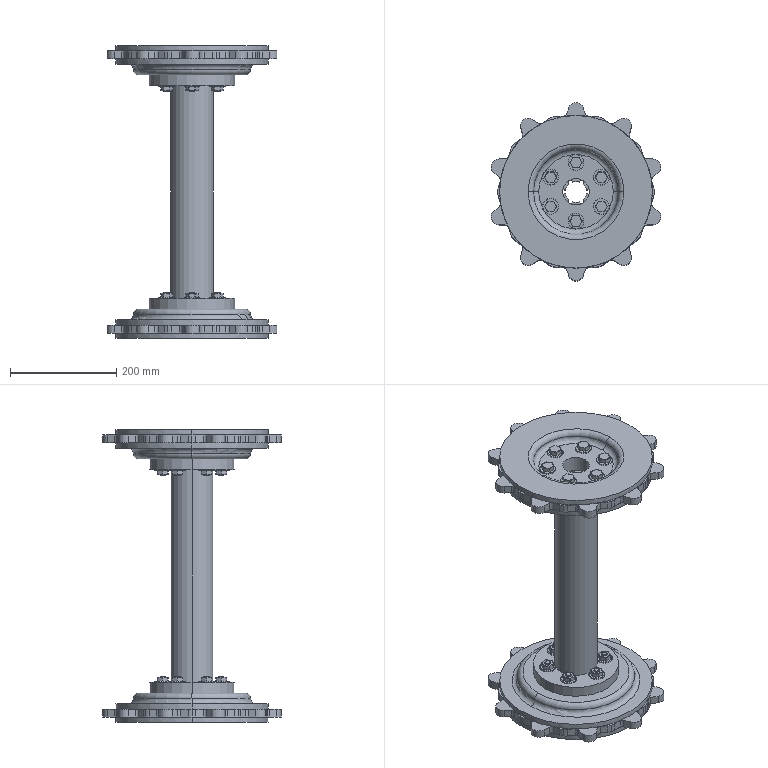Part | SolidWorks | 27 solids | 1698 faces | box 319.348 x 334.309 x 550 mm | volume 7592886 mm3 | cylinder 860 | plane 414 | sphere 288 | cone 72 | torus 64 | commonest cylinder face diameters 1 x288 2 x288 10 x72 30 x48 12 x40 48 x40